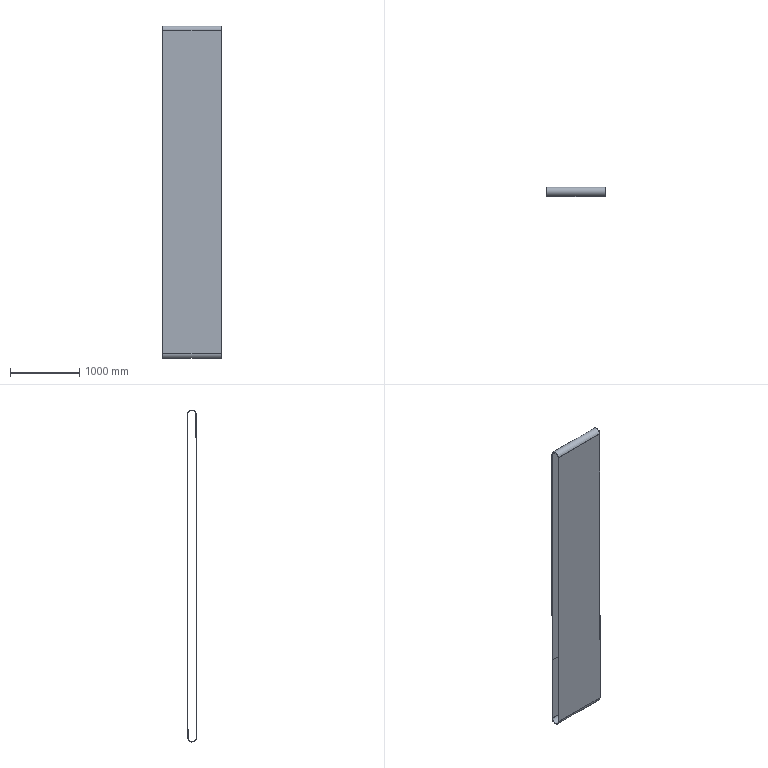Part | SolidWorks | features Extrusion 1 | 1 solid | 16 faces | box 850 x 135 x 4803 mm | volume 41389503 mm3 | cylinder 8 | plane 8 | commonest cylinder face diameters 120 x4 130 x4
STEP:
#1=CARTESIAN_POINT('',(-428.6,-104.4,394.));
#2=VERTEX_POINT('',#1);
#3=CARTESIAN_POINT('',(-428.6,-224.4,394.064));
#4=VERTEX_POINT('',#3);
#5=CARTESIAN_POINT('',(-428.6,-164.4,394.));
#6=DIRECTION('',(1.,0.,0.));
#7=DIRECTION('',(0.,-1.,0.));
#8=AXIS2_PLACEMENT_3D('',#5,#6,#7);
#9=CIRCLE('',#8,60.);
#10=EDGE_CURVE('',#2,#4,#9,.T.);
#11=ORIENTED_EDGE('',*,*,#10,.F.);
#12=CARTESIAN_POINT('',(421.4,-104.4,394.));
#13=VERTEX_POINT('',#12);
#14=CARTESIAN_POINT('',(-5233.497,-104.4,394.));
#15=DIRECTION('',(1.,0.,0.));
#16=VECTOR('',#15,1000.);
#17=LINE('',#14,#16);
#18=EDGE_CURVE('',#2,#13,#17,.T.);
#19=ORIENTED_EDGE('',*,*,#18,.T.);
#20=CARTESIAN_POINT('',(421.4,-224.4,394.064));
#21=VERTEX_POINT('',#20);
#22=CARTESIAN_POINT('',(421.4,-164.4,394.));
#23=DIRECTION('',(1.,0.,0.));
#24=DIRECTION('',(0.,1.,0.));
#25=AXIS2_PLACEMENT_3D('',#22,#23,#24);
#26=CIRCLE('',#25,60.);
#27=EDGE_CURVE('',#13,#21,#26,.T.);
#28=ORIENTED_EDGE('',*,*,#27,.T.);
#29=CARTESIAN_POINT('',(-5233.497,-224.4,394.064));
#30=DIRECTION('',(1.,0.,0.));
#31=VECTOR('',#30,1000.);
#32=LINE('',#29,#31);
#33=EDGE_CURVE('',#4,#21,#32,.T.);
#34=ORIENTED_EDGE('',*,*,#33,.F.);
#35=EDGE_LOOP('',(#11,#19,#28,#34));
#36=FACE_OUTER_BOUND('',#35,.T.);
#37=CARTESIAN_POINT('',(-5233.497,-164.4,394.));
#38=DIRECTION('',(1.,0.,0.));
#39=DIRECTION('',(0.,1.,0.));
#40=AXIS2_PLACEMENT_3D('',#37,#38,#39);
#41=CYLINDRICAL_SURFACE('',#40,60.);
#42=ADVANCED_FACE('',(#36),#41,.F.);
#43=CARTESIAN_POINT('',(-428.6,-99.4,393.964));
#44=VERTEX_POINT('',#43);
#45=CARTESIAN_POINT('',(-428.6,-99.4,394.));
#46=VERTEX_POINT('',#45);
#47=CARTESIAN_POINT('',(-428.6,-164.4,394.));
#48=DIRECTION('',(1.,0.,0.));
#49=DIRECTION('',(0.,-1.,0.));
#50=AXIS2_PLACEMENT_3D('',#47,#48,#49);
#51=CIRCLE('',#50,65.);
#52=EDGE_CURVE('',#44,#46,#51,.T.);
#53=ORIENTED_EDGE('',*,*,#52,.T.);
#54=CARTESIAN_POINT('',(421.4,-99.4,394.));
#55=VERTEX_POINT('',#54);
#56=CARTESIAN_POINT('',(-5233.497,-99.4,394.));
#57=DIRECTION('',(1.,0.,0.));
#58=VECTOR('',#57,1000.);
#59=LINE('',#56,#58);
#60=EDGE_CURVE('',#46,#55,#59,.T.);
#61=ORIENTED_EDGE('',*,*,#60,.T.);
#62=CARTESIAN_POINT('',(421.4,-99.4,393.964));
#63=VERTEX_POINT('',#62);
#64=CARTESIAN_POINT('',(421.4,-164.4,394.));
#65=DIRECTION('',(1.,0.,0.));
#66=DIRECTION('',(0.,1.,0.));
#67=AXIS2_PLACEMENT_3D('',#64,#65,#66);
#68=CIRCLE('',#67,65.);
#69=EDGE_CURVE('',#63,#55,#68,.T.);
#70=ORIENTED_EDGE('',*,*,#69,.F.);
#71=CARTESIAN_POINT('',(-5233.497,-99.4,393.964));
#72=DIRECTION('',(1.,0.,0.));
#73=VECTOR('',#72,1000.);
#74=LINE('',#71,#73);
#75=EDGE_CURVE('',#44,#63,#74,.T.);
#76=ORIENTED_EDGE('',*,*,#75,.F.);
#77=EDGE_LOOP('',(#53,#61,#70,#76));
#78=FACE_OUTER_BOUND('',#77,.T.);
#79=CARTESIAN_POINT('',(-5233.497,-164.4,394.));
#80=DIRECTION('',(1.,0.,0.));
#81=DIRECTION('',(0.,1.,0.));
#82=AXIS2_PLACEMENT_3D('',#79,#80,#81);
#83=CYLINDRICAL_SURFACE('',#82,65.);
#84=ADVANCED_FACE('',(#78),#83,.T.);
#85=ORIENTED_EDGE('',*,*,#60,.F.);
#86=CARTESIAN_POINT('',(-428.6,-229.4,394.07));
#87=VERTEX_POINT('',#86);
#88=CARTESIAN_POINT('',(-428.6,-164.4,394.));
#89=DIRECTION('',(1.,0.,0.));
#90=DIRECTION('',(0.,-1.,0.));
#91=AXIS2_PLACEMENT_3D('',#88,#89,#90);
#92=CIRCLE('',#91,65.);
#93=EDGE_CURVE('',#46,#87,#92,.T.);
#94=ORIENTED_EDGE('',*,*,#93,.T.);
#95=CARTESIAN_POINT('',(421.4,-229.4,394.07));
#96=VERTEX_POINT('',#95);
#97=CARTESIAN_POINT('',(-5233.497,-229.4,394.07));
#98=DIRECTION('',(1.,0.,0.));
#99=VECTOR('',#98,1000.);
#100=LINE('',#97,#99);
#101=EDGE_CURVE('',#87,#96,#100,.T.);
#102=ORIENTED_EDGE('',*,*,#101,.T.);
#103=CARTESIAN_POINT('',(421.4,-164.4,394.));
#104=DIRECTION('',(1.,0.,0.));
#105=DIRECTION('',(0.,1.,0.));
#106=AXIS2_PLACEMENT_3D('',#103,#104,#105);
#107=CIRCLE('',#106,65.);
#108=EDGE_CURVE('',#55,#96,#107,.T.);
#109=ORIENTED_EDGE('',*,*,#108,.F.);
#110=EDGE_LOOP('',(#85,#94,#102,#109));
#111=FACE_OUTER_BOUND('',#110,.T.);
#112=CARTESIAN_POINT('',(-5233.497,-164.4,394.));
#113=DIRECTION('',(1.,0.,0.));
#114=DIRECTION('',(0.,1.,0.));
#115=AXIS2_PLACEMENT_3D('',#112,#113,#114);
#116=CYLINDRICAL_SURFACE('',#115,65.);
#117=ADVANCED_FACE('',(#111),#116,.T.);
#118=CARTESIAN_POINT('',(-428.6,-101.4,-3251.036));
#119=VERTEX_POINT('',#118);
#120=CARTESIAN_POINT('',(421.4,-101.4,-3251.036));
#121=VERTEX_POINT('',#120);
#122=CARTESIAN_POINT('',(-5233.497,-101.4,-3251.036));
#123=DIRECTION('',(1.,0.,0.));
#124=VECTOR('',#123,1000.);
#125=LINE('',#122,#124);
#126=EDGE_CURVE('',#119,#121,#125,.T.);
#127=ORIENTED_EDGE('',*,*,#126,.F.);
#128=CARTESIAN_POINT('',(-428.6,-99.4,393.964));
#129=DIRECTION('',(0.,0.0005487,1.));
#130=VECTOR('',#129,1000.);
#131=LINE('',#128,#130);
#132=EDGE_CURVE('',#119,#44,#131,.T.);
#133=ORIENTED_EDGE('',*,*,#132,.T.);
#134=ORIENTED_EDGE('',*,*,#75,.T.);
#135=CARTESIAN_POINT('',(421.4,-99.4,393.964));
#136=DIRECTION('',(0.,0.0005487,1.));
#137=VECTOR('',#136,1000.);
#138=LINE('',#135,#137);
#139=EDGE_CURVE('',#121,#63,#138,.T.);
#140=ORIENTED_EDGE('',*,*,#139,.F.);
#141=EDGE_LOOP('',(#127,#133,#134,#140));
#142=FACE_OUTER_BOUND('',#141,.T.);
#143=CARTESIAN_POINT('',(-5233.497,-99.4,393.964));
#144=DIRECTION('',(0.,1.,-0.0005487));
#145=DIRECTION('',(0.,0.0005487,1.));
#146=AXIS2_PLACEMENT_3D('',#143,#144,#145);
#147=PLANE('',#146);
#148=ADVANCED_FACE('',(#142),#147,.T.);
#149=CARTESIAN_POINT('',(-428.6,-101.4,-3251.19));
#150=VERTEX_POINT('',#149);
#151=CARTESIAN_POINT('',(421.4,-101.4,-3251.19));
#152=VERTEX_POINT('',#151);
#153=CARTESIAN_POINT('',(-5233.497,-101.4,-3251.19));
#154=DIRECTION('',(1.,0.,0.));
#155=VECTOR('',#154,1000.);
#156=LINE('',#153,#155);
#157=EDGE_CURVE('',#150,#152,#156,.T.);
#158=ORIENTED_EDGE('',*,*,#157,.F.);
#159=CARTESIAN_POINT('',(-428.6,-166.4,-3251.));
#160=DIRECTION('',(1.,0.,0.));
#161=DIRECTION('',(0.,-1.,0.));
#162=AXIS2_PLACEMENT_3D('',#159,#160,#161);
#163=CIRCLE('',#162,65.);
#164=EDGE_CURVE('',#150,#119,#163,.T.);
#165=ORIENTED_EDGE('',*,*,#164,.T.);
#166=ORIENTED_EDGE('',*,*,#126,.T.);
#167=CARTESIAN_POINT('',(421.4,-166.4,-3251.));
#168=DIRECTION('',(1.,0.,0.));
#169=DIRECTION('',(0.,1.,0.));
#170=AXIS2_PLACEMENT_3D('',#167,#168,#169);
#171=CIRCLE('',#170,65.);
#172=EDGE_CURVE('',#152,#121,#171,.T.);
#173=ORIENTED_EDGE('',*,*,#172,.F.);
#174=EDGE_LOOP('',(#158,#165,#166,#173));
#175=FACE_OUTER_BOUND('',#174,.T.);
#176=CARTESIAN_POINT('',(-5233.497,-166.4,-3251.));
#177=DIRECTION('',(1.,0.,0.));
#178=DIRECTION('',(0.,1.,0.));
#179=AXIS2_PLACEMENT_3D('',#176,#177,#178);
#180=CYLINDRICAL_SURFACE('',#179,65.);
#181=ADVANCED_FACE('',(#175),#180,.T.);
#182=CARTESIAN_POINT('',(-428.6,-104.4,-4279.19));
#183=VERTEX_POINT('',#182);
#184=CARTESIAN_POINT('',(421.4,-104.4,-4279.19));
#185=VERTEX_POINT('',#184);
#186=CARTESIAN_POINT('',(-5233.497,-104.4,-4279.19));
#187=DIRECTION('',(1.,0.,0.));
#188=VECTOR('',#187,1000.);
#189=LINE('',#186,#188);
#190=EDGE_CURVE('',#183,#185,#189,.T.);
#191=ORIENTED_EDGE('',*,*,#190,.F.);
#192=CARTESIAN_POINT('',(-428.6,-101.4,-3251.19));
#193=DIRECTION('',(0.,0.002918,1.));
#194=VECTOR('',#193,1000.);
#195=LINE('',#192,#194);
#196=EDGE_CURVE('',#183,#150,#195,.T.);
#197=ORIENTED_EDGE('',*,*,#196,.T.);
#198=ORIENTED_EDGE('',*,*,#157,.T.);
#199=CARTESIAN_POINT('',(421.4,-101.4,-3251.19));
#200=DIRECTION('',(0.,0.002918,1.));
#201=VECTOR('',#200,1000.);
#202=LINE('',#199,#201);
#203=EDGE_CURVE('',#185,#152,#202,.T.);
#204=ORIENTED_EDGE('',*,*,#203,.F.);
#205=EDGE_LOOP('',(#191,#197,#198,#204));
#206=FACE_OUTER_BOUND('',#205,.T.);
#207=CARTESIAN_POINT('',(-5233.497,-101.4,-3251.19));
#208=DIRECTION('',(0.,1.,-0.002918));
#209=DIRECTION('',(0.,0.002918,1.));
#210=AXIS2_PLACEMENT_3D('',#207,#208,#209);
#211=PLANE('',#210);
#212=ADVANCED_FACE('',(#206),#211,.T.);
#213=CARTESIAN_POINT('',(-428.6,-234.4,-4278.93));
#214=VERTEX_POINT('',#213);
#215=CARTESIAN_POINT('',(421.4,-234.4,-4278.93));
#216=VERTEX_POINT('',#215);
#217=CARTESIAN_POINT('',(-5233.497,-234.4,-4278.93));
#218=DIRECTION('',(1.,0.,0.));
#219=VECTOR('',#218,1000.);
#220=LINE('',#217,#219);
#221=EDGE_CURVE('',#214,#216,#220,.T.);
#222=ORIENTED_EDGE('',*,*,#221,.F.);
#223=CARTESIAN_POINT('',(-428.6,-169.4,-4279.));
#224=DIRECTION('',(1.,0.,0.));
#225=DIRECTION('',(0.,-1.,0.));
#226=AXIS2_PLACEMENT_3D('',#223,#224,#225);
#227=CIRCLE('',#226,65.);
#228=EDGE_CURVE('',#214,#183,#227,.T.);
#229=ORIENTED_EDGE('',*,*,#228,.T.);
#230=ORIENTED_EDGE('',*,*,#190,.T.);
#231=CARTESIAN_POINT('',(421.4,-169.4,-4279.));
#232=DIRECTION('',(1.,0.,0.));
#233=DIRECTION('',(0.,1.,0.));
#234=AXIS2_PLACEMENT_3D('',#231,#232,#233);
#235=CIRCLE('',#234,65.);
#236=EDGE_CURVE('',#216,#185,#235,.T.);
#237=ORIENTED_EDGE('',*,*,#236,.F.);
#238=EDGE_LOOP('',(#222,#229,#230,#237));
#239=FACE_OUTER_BOUND('',#238,.T.);
#240=CARTESIAN_POINT('',(-5233.497,-169.4,-4279.));
#241=DIRECTION('',(1.,0.,0.));
#242=DIRECTION('',(0.,1.,0.));
#243=AXIS2_PLACEMENT_3D('',#240,#241,#242);
#244=CYLINDRICAL_SURFACE('',#243,65.);
#245=ADVANCED_FACE('',(#239),#244,.T.);
#246=ORIENTED_EDGE('',*,*,#101,.F.);
#247=CARTESIAN_POINT('',(-428.6,-229.4,394.07));
#248=DIRECTION('',(0.,-0.00107,-1.));
#249=VECTOR('',#248,1000.);
#250=LINE('',#247,#249);
#251=EDGE_CURVE('',#87,#214,#250,.T.);
#252=ORIENTED_EDGE('',*,*,#251,.T.);
#253=ORIENTED_EDGE('',*,*,#221,.T.);
#254=CARTESIAN_POINT('',(421.4,-229.4,394.07));
#255=DIRECTION('',(0.,-0.00107,-1.));
#256=VECTOR('',#255,1000.);
#257=LINE('',#254,#256);
#258=EDGE_CURVE('',#96,#216,#257,.T.);
#259=ORIENTED_EDGE('',*,*,#258,.F.);
#260=EDGE_LOOP('',(#246,#252,#253,#259));
#261=FACE_OUTER_BOUND('',#260,.T.);
#262=CARTESIAN_POINT('',(-5233.497,-229.4,394.07));
#263=DIRECTION('',(0.,-1.,0.00107));
#264=DIRECTION('',(0.,-0.00107,-1.));
#265=AXIS2_PLACEMENT_3D('',#262,#263,#264);
#266=PLANE('',#265);
#267=ADVANCED_FACE('',(#261),#266,.T.);
#268=ORIENTED_EDGE('',*,*,#18,.F.);
#269=CARTESIAN_POINT('',(-428.6,-104.4,393.967));
#270=VERTEX_POINT('',#269);
#271=CARTESIAN_POINT('',(-428.6,-164.4,394.));
#272=DIRECTION('',(1.,0.,0.));
#273=DIRECTION('',(0.,-1.,0.));
#274=AXIS2_PLACEMENT_3D('',#271,#272,#273);
#275=CIRCLE('',#274,60.);
#276=EDGE_CURVE('',#270,#2,#275,.T.);
#277=ORIENTED_EDGE('',*,*,#276,.F.);
#278=CARTESIAN_POINT('',(421.4,-104.4,393.967));
#279=VERTEX_POINT('',#278);
#280=CARTESIAN_POINT('',(-5233.497,-104.4,393.967));
#281=DIRECTION('',(1.,0.,0.));
#282=VECTOR('',#281,1000.);
#283=LINE('',#280,#282);
#284=EDGE_CURVE('',#270,#279,#283,.T.);
#285=ORIENTED_EDGE('',*,*,#284,.T.);
#286=CARTESIAN_POINT('',(421.4,-164.4,394.));
#287=DIRECTION('',(1.,0.,0.));
#288=DIRECTION('',(0.,1.,0.));
#289=AXIS2_PLACEMENT_3D('',#286,#287,#288);
#290=CIRCLE('',#289,60.);
#291=EDGE_CURVE('',#279,#13,#290,.T.);
#292=ORIENTED_EDGE('',*,*,#291,.T.);
#293=EDGE_LOOP('',(#268,#277,#285,#292));
#294=FACE_OUTER_BOUND('',#293,.T.);
#295=CARTESIAN_POINT('',(-5233.497,-164.4,394.));
#296=DIRECTION('',(1.,0.,0.));
#297=DIRECTION('',(0.,1.,0.));
#298=AXIS2_PLACEMENT_3D('',#295,#296,#297);
#299=CYLINDRICAL_SURFACE('',#298,60.);
#300=ADVANCED_FACE('',(#294),#299,.F.);
#301=CARTESIAN_POINT('',(-428.6,-106.4,-3251.033));
#302=VERTEX_POINT('',#301);
#303=CARTESIAN_POINT('',(-428.6,-104.4,393.967));
#304=DIRECTION('',(0.,0.0005487,1.));
#305=VECTOR('',#304,1000.);
#306=LINE('',#303,#305);
#307=EDGE_CURVE('',#302,#270,#306,.T.);
#308=ORIENTED_EDGE('',*,*,#307,.F.);
#309=CARTESIAN_POINT('',(421.4,-106.4,-3251.033));
#310=VERTEX_POINT('',#309);
#311=CARTESIAN_POINT('',(-5233.497,-106.4,-3251.033));
#312=DIRECTION('',(1.,0.,0.));
#313=VECTOR('',#312,1000.);
#314=LINE('',#311,#313);
#315=EDGE_CURVE('',#302,#310,#314,.T.);
#316=ORIENTED_EDGE('',*,*,#315,.T.);
#317=CARTESIAN_POINT('',(421.4,-104.4,393.967));
#318=DIRECTION('',(0.,0.0005487,1.));
#319=VECTOR('',#318,1000.);
#320=LINE('',#317,#319);
#321=EDGE_CURVE('',#310,#279,#320,.T.);
#322=ORIENTED_EDGE('',*,*,#321,.T.);
#323=ORIENTED_EDGE('',*,*,#284,.F.);
#324=EDGE_LOOP('',(#308,#316,#322,#323));
#325=FACE_OUTER_BOUND('',#324,.T.);
#326=CARTESIAN_POINT('',(-5233.497,-104.4,393.967));
#327=DIRECTION('',(0.,1.,-0.0005487));
#328=DIRECTION('',(0.,0.0005487,1.));
#329=AXIS2_PLACEMENT_3D('',#326,#327,#328);
#330=PLANE('',#329);
#331=ADVANCED_FACE('',(#325),#330,.F.);
#332=CARTESIAN_POINT('',(-428.6,-106.4,-3251.175));
#333=VERTEX_POINT('',#332);
#334=CARTESIAN_POINT('',(-428.6,-166.4,-3251.));
#335=DIRECTION('',(1.,0.,0.));
#336=DIRECTION('',(0.,-1.,0.));
#337=AXIS2_PLACEMENT_3D('',#334,#335,#336);
#338=CIRCLE('',#337,60.);
#339=EDGE_CURVE('',#333,#302,#338,.T.);
#340=ORIENTED_EDGE('',*,*,#339,.F.);
#341=CARTESIAN_POINT('',(421.4,-106.4,-3251.175));
#342=VERTEX_POINT('',#341);
#343=CARTESIAN_POINT('',(-5233.497,-106.4,-3251.175));
#344=DIRECTION('',(1.,0.,0.));
#345=VECTOR('',#344,1000.);
#346=LINE('',#343,#345);
#347=EDGE_CURVE('',#333,#342,#346,.T.);
#348=ORIENTED_EDGE('',*,*,#347,.T.);
#349=CARTESIAN_POINT('',(421.4,-166.4,-3251.));
#350=DIRECTION('',(1.,0.,0.));
#351=DIRECTION('',(0.,1.,0.));
#352=AXIS2_PLACEMENT_3D('',#349,#350,#351);
#353=CIRCLE('',#352,60.);
#354=EDGE_CURVE('',#342,#310,#353,.T.);
#355=ORIENTED_EDGE('',*,*,#354,.T.);
#356=ORIENTED_EDGE('',*,*,#315,.F.);
#357=EDGE_LOOP('',(#340,#348,#355,#356));
#358=FACE_OUTER_BOUND('',#357,.T.);
#359=CARTESIAN_POINT('',(-5233.497,-166.4,-3251.));
#360=DIRECTION('',(1.,0.,0.));
#361=DIRECTION('',(0.,1.,0.));
#362=AXIS2_PLACEMENT_3D('',#359,#360,#361);
#363=CYLINDRICAL_SURFACE('',#362,60.);
#364=ADVANCED_FACE('',(#358),#363,.F.);
#365=CARTESIAN_POINT('',(-428.6,-109.4,-4279.175));
#366=VERTEX_POINT('',#365);
#367=CARTESIAN_POINT('',(-428.6,-106.4,-3251.175));
#368=DIRECTION('',(0.,0.002918,1.));
#369=VECTOR('',#368,1000.);
#370=LINE('',#367,#369);
#371=EDGE_CURVE('',#366,#333,#370,.T.);
#372=ORIENTED_EDGE('',*,*,#371,.F.);
#373=CARTESIAN_POINT('',(421.4,-109.4,-4279.175));
#374=VERTEX_POINT('',#373);
#375=CARTESIAN_POINT('',(-5233.497,-109.4,-4279.175));
#376=DIRECTION('',(1.,0.,0.));
#377=VECTOR('',#376,1000.);
#378=LINE('',#375,#377);
#379=EDGE_CURVE('',#366,#374,#378,.T.);
#380=ORIENTED_EDGE('',*,*,#379,.T.);
#381=CARTESIAN_POINT('',(421.4,-106.4,-3251.175));
#382=DIRECTION('',(0.,0.002918,1.));
#383=VECTOR('',#382,1000.);
#384=LINE('',#381,#383);
#385=EDGE_CURVE('',#374,#342,#384,.T.);
#386=ORIENTED_EDGE('',*,*,#385,.T.);
#387=ORIENTED_EDGE('',*,*,#347,.F.);
#388=EDGE_LOOP('',(#372,#380,#386,#387));
#389=FACE_OUTER_BOUND('',#388,.T.);
#390=CARTESIAN_POINT('',(-5233.497,-106.4,-3251.175));
#391=DIRECTION('',(0.,1.,-0.002918));
#392=DIRECTION('',(0.,0.002918,1.));
#393=AXIS2_PLACEMENT_3D('',#390,#391,#392);
#394=PLANE('',#393);
#395=ADVANCED_FACE('',(#389),#394,.F.);
#396=CARTESIAN_POINT('',(-428.6,-229.4,-4278.936));
#397=VERTEX_POINT('',#396);
#398=CARTESIAN_POINT('',(-428.6,-169.4,-4279.));
#399=DIRECTION('',(1.,0.,0.));
#400=DIRECTION('',(0.,-1.,0.));
#401=AXIS2_PLACEMENT_3D('',#398,#399,#400);
#402=CIRCLE('',#401,60.);
#403=EDGE_CURVE('',#397,#366,#402,.T.);
#404=ORIENTED_EDGE('',*,*,#403,.F.);
#405=CARTESIAN_POINT('',(421.4,-229.4,-4278.936));
#406=VERTEX_POINT('',#405);
#407=CARTESIAN_POINT('',(-5233.497,-229.4,-4278.936));
#408=DIRECTION('',(1.,0.,0.));
#409=VECTOR('',#408,1000.);
#410=LINE('',#407,#409);
#411=EDGE_CURVE('',#397,#406,#410,.T.);
#412=ORIENTED_EDGE('',*,*,#411,.T.);
#413=CARTESIAN_POINT('',(421.4,-169.4,-4279.));
#414=DIRECTION('',(1.,0.,0.));
#415=DIRECTION('',(0.,1.,0.));
#416=AXIS2_PLACEMENT_3D('',#413,#414,#415);
#417=CIRCLE('',#416,60.);
#418=EDGE_CURVE('',#406,#374,#417,.T.);
#419=ORIENTED_EDGE('',*,*,#418,.T.);
#420=ORIENTED_EDGE('',*,*,#379,.F.);
#421=EDGE_LOOP('',(#404,#412,#419,#420));
#422=FACE_OUTER_BOUND('',#421,.T.);
#423=CARTESIAN_POINT('',(-5233.497,-169.4,-4279.));
#424=DIRECTION('',(1.,0.,0.));
#425=DIRECTION('',(0.,1.,0.));
#426=AXIS2_PLACEMENT_3D('',#423,#424,#425);
#427=CYLINDRICAL_SURFACE('',#426,60.);
#428=ADVANCED_FACE('',(#422),#427,.F.);
#429=CARTESIAN_POINT('',(-428.6,-224.4,394.064));
#430=DIRECTION('',(0.,-0.00107,-1.));
#431=VECTOR('',#430,1000.);
#432=LINE('',#429,#431);
#433=EDGE_CURVE('',#4,#397,#432,.T.);
#434=ORIENTED_EDGE('',*,*,#433,.F.);
#435=ORIENTED_EDGE('',*,*,#33,.T.);
#436=CARTESIAN_POINT('',(421.4,-224.4,394.064));
#437=DIRECTION('',(0.,-0.00107,-1.));
#438=VECTOR('',#437,1000.);
#439=LINE('',#436,#438);
#440=EDGE_CURVE('',#21,#406,#439,.T.);
#441=ORIENTED_EDGE('',*,*,#440,.T.);
#442=ORIENTED_EDGE('',*,*,#411,.F.);
#443=EDGE_LOOP('',(#434,#435,#441,#442));
#444=FACE_OUTER_BOUND('',#443,.T.);
#445=CARTESIAN_POINT('',(-5233.497,-224.4,394.064));
#446=DIRECTION('',(0.,-1.,0.00107));
#447=DIRECTION('',(0.,-0.00107,-1.));
#448=AXIS2_PLACEMENT_3D('',#445,#446,#447);
#449=PLANE('',#448);
#450=ADVANCED_FACE('',(#444),#449,.F.);
#451=ORIENTED_EDGE('',*,*,#291,.F.);
#452=ORIENTED_EDGE('',*,*,#321,.F.);
#453=ORIENTED_EDGE('',*,*,#354,.F.);
#454=ORIENTED_EDGE('',*,*,#385,.F.);
#455=ORIENTED_EDGE('',*,*,#418,.F.);
#456=ORIENTED_EDGE('',*,*,#440,.F.);
#457=ORIENTED_EDGE('',*,*,#27,.F.);
#458=EDGE_LOOP('',(#451,#452,#453,#454,#455,#456,#457));
#459=FACE_BOUND('',#458,.T.);
#460=ORIENTED_EDGE('',*,*,#69,.T.);
#461=ORIENTED_EDGE('',*,*,#108,.T.);
#462=ORIENTED_EDGE('',*,*,#258,.T.);
#463=ORIENTED_EDGE('',*,*,#236,.T.);
#464=ORIENTED_EDGE('',*,*,#203,.T.);
#465=ORIENTED_EDGE('',*,*,#172,.T.);
#466=ORIENTED_EDGE('',*,*,#139,.T.);
#467=EDGE_LOOP('',(#460,#461,#462,#463,#464,#465,#466));
#468=FACE_OUTER_BOUND('',#467,.T.);
#469=CARTESIAN_POINT('',(421.4,-164.4,394.));
#470=DIRECTION('',(1.,0.,0.));
#471=DIRECTION('',(0.,1.,0.));
#472=AXIS2_PLACEMENT_3D('',#469,#470,#471);
#473=PLANE('',#472);
#474=ADVANCED_FACE('',(#459,#468),#473,.T.);
#475=ORIENTED_EDGE('',*,*,#52,.F.);
#476=ORIENTED_EDGE('',*,*,#132,.F.);
#477=ORIENTED_EDGE('',*,*,#164,.F.);
#478=ORIENTED_EDGE('',*,*,#196,.F.);
#479=ORIENTED_EDGE('',*,*,#228,.F.);
#480=ORIENTED_EDGE('',*,*,#251,.F.);
#481=ORIENTED_EDGE('',*,*,#93,.F.);
#482=EDGE_LOOP('',(#475,#476,#477,#478,#479,#480,#481));
#483=FACE_OUTER_BOUND('',#482,.T.);
#484=ORIENTED_EDGE('',*,*,#307,.T.);
#485=ORIENTED_EDGE('',*,*,#276,.T.);
#486=ORIENTED_EDGE('',*,*,#10,.T.);
#487=ORIENTED_EDGE('',*,*,#433,.T.);
#488=ORIENTED_EDGE('',*,*,#403,.T.);
#489=ORIENTED_EDGE('',*,*,#371,.T.);
#490=ORIENTED_EDGE('',*,*,#339,.T.);
#491=EDGE_LOOP('',(#484,#485,#486,#487,#488,#489,#490));
#492=FACE_BOUND('',#491,.T.);
#493=CARTESIAN_POINT('',(-428.6,-144.941,389.38));
#494=DIRECTION('',(-1.,0.,0.));
#495=DIRECTION('',(0.,-0.973,0.231));
#496=AXIS2_PLACEMENT_3D('',#493,#494,#495);
#497=PLANE('',#496);
#498=ADVANCED_FACE('',(#483,#492),#497,.T.);
#499=CLOSED_SHELL('',(#42,#84,#117,#148,#181,#212,#245,#267,#300,#331,#364,#395,#428,#450,#474,#498));
#500=MANIFOLD_SOLID_BREP('',#499);
#501=CARTESIAN_POINT('',(0.,0.,0.));
#502=DIRECTION('',(0.,0.,1.));
#503=DIRECTION('',(1.,0.,0.));
#504=AXIS2_PLACEMENT_3D('',#501,#502,#503);
#505=(LENGTH_UNIT()NAMED_UNIT(*)SI_UNIT(.MILLI.,.METRE.));
#506=UNCERTAINTY_MEASURE_WITH_UNIT(LENGTH_MEASURE(0.00001),#505,'','');
#507=(NAMED_UNIT(*)PLANE_ANGLE_UNIT()SI_UNIT($,.RADIAN.));
#508=(NAMED_UNIT(*)SI_UNIT($,.STERADIAN.)SOLID_ANGLE_UNIT());
#509=(GEOMETRIC_REPRESENTATION_CONTEXT(3)GLOBAL_UNCERTAINTY_ASSIGNED_CONTEXT((#506))GLOBAL_UNIT_ASSIGNED_CONTEXT((#505,#507,#508))REPRESENTATION_CONTEXT('',''));
#510=ADVANCED_BREP_SHAPE_REPRESENTATION('',(#500,#504),#509);